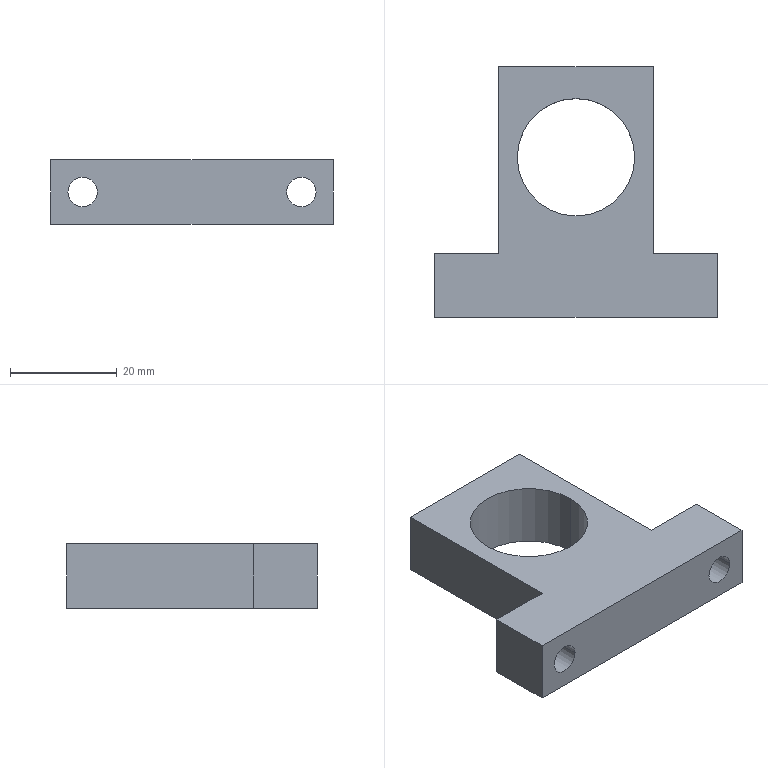Part | SolidWorks | features ICE 2, Extrusion 1 | 1 solid | 22 faces | box 53 x 47 x 12 mm | volume 14045 mm3 | plane 12 | cylinder 10 | commonest cylinder face diameters 5.5 x4 10 x4 22 x2
STEP:
#1=CARTESIAN_POINT('',(-5.27,-9.838,6.));
#2=VERTEX_POINT('',#1);
#3=CARTESIAN_POINT('',(-15.27,-9.838,6.));
#4=VERTEX_POINT('',#3);
#5=CARTESIAN_POINT('',(-10.27,-9.838,6.));
#6=DIRECTION('',(0.,1.,0.));
#7=DIRECTION('',(-1.,0.,0.));
#8=AXIS2_PLACEMENT_3D('',#5,#6,#7);
#9=CIRCLE('',#8,5.);
#10=EDGE_CURVE('',#2,#4,#9,.T.);
#11=ORIENTED_EDGE('',*,*,#10,.F.);
#12=CARTESIAN_POINT('',(-5.27,-4.038,6.));
#13=VERTEX_POINT('',#12);
#14=CARTESIAN_POINT('',(-5.27,-9.838,6.));
#15=DIRECTION('',(0.,1.,0.));
#16=VECTOR('',#15,1000.);
#17=LINE('',#14,#16);
#18=EDGE_CURVE('',#2,#13,#17,.T.);
#19=ORIENTED_EDGE('',*,*,#18,.T.);
#20=CARTESIAN_POINT('',(-15.27,-4.038,6.));
#21=VERTEX_POINT('',#20);
#22=CARTESIAN_POINT('',(-10.27,-4.038,6.));
#23=DIRECTION('',(0.,1.,0.));
#24=DIRECTION('',(-1.,0.,0.));
#25=AXIS2_PLACEMENT_3D('',#22,#23,#24);
#26=CIRCLE('',#25,5.);
#27=EDGE_CURVE('',#13,#21,#26,.T.);
#28=ORIENTED_EDGE('',*,*,#27,.T.);
#29=CARTESIAN_POINT('',(-15.27,-9.838,6.));
#30=DIRECTION('',(0.,1.,0.));
#31=VECTOR('',#30,1000.);
#32=LINE('',#29,#31);
#33=EDGE_CURVE('',#4,#21,#32,.T.);
#34=ORIENTED_EDGE('',*,*,#33,.F.);
#35=EDGE_LOOP('',(#11,#19,#28,#34));
#36=FACE_OUTER_BOUND('',#35,.T.);
#37=CARTESIAN_POINT('',(-10.27,-9.838,6.));
#38=DIRECTION('',(0.,1.,0.));
#39=DIRECTION('',(-1.,0.,0.));
#40=AXIS2_PLACEMENT_3D('',#37,#38,#39);
#41=CYLINDRICAL_SURFACE('',#40,5.);
#42=ADVANCED_FACE('',(#36),#41,.F.);
#43=CARTESIAN_POINT('',(35.73,-9.838,6.));
#44=VERTEX_POINT('',#43);
#45=CARTESIAN_POINT('',(25.73,-9.838,6.));
#46=VERTEX_POINT('',#45);
#47=CARTESIAN_POINT('',(30.73,-9.838,6.));
#48=DIRECTION('',(0.,1.,0.));
#49=DIRECTION('',(-1.,0.,0.));
#50=AXIS2_PLACEMENT_3D('',#47,#48,#49);
#51=CIRCLE('',#50,5.);
#52=EDGE_CURVE('',#44,#46,#51,.T.);
#53=ORIENTED_EDGE('',*,*,#52,.F.);
#54=CARTESIAN_POINT('',(35.73,-4.038,6.));
#55=VERTEX_POINT('',#54);
#56=CARTESIAN_POINT('',(35.73,-9.838,6.));
#57=DIRECTION('',(0.,1.,0.));
#58=VECTOR('',#57,1000.);
#59=LINE('',#56,#58);
#60=EDGE_CURVE('',#44,#55,#59,.T.);
#61=ORIENTED_EDGE('',*,*,#60,.T.);
#62=CARTESIAN_POINT('',(25.73,-4.038,6.));
#63=VERTEX_POINT('',#62);
#64=CARTESIAN_POINT('',(30.73,-4.038,6.));
#65=DIRECTION('',(0.,1.,0.));
#66=DIRECTION('',(-1.,0.,0.));
#67=AXIS2_PLACEMENT_3D('',#64,#65,#66);
#68=CIRCLE('',#67,5.);
#69=EDGE_CURVE('',#55,#63,#68,.T.);
#70=ORIENTED_EDGE('',*,*,#69,.T.);
#71=CARTESIAN_POINT('',(25.73,-9.838,6.));
#72=DIRECTION('',(0.,1.,0.));
#73=VECTOR('',#72,1000.);
#74=LINE('',#71,#73);
#75=EDGE_CURVE('',#46,#63,#74,.T.);
#76=ORIENTED_EDGE('',*,*,#75,.F.);
#77=EDGE_LOOP('',(#53,#61,#70,#76));
#78=FACE_OUTER_BOUND('',#77,.T.);
#79=CARTESIAN_POINT('',(30.73,-9.838,6.));
#80=DIRECTION('',(0.,1.,0.));
#81=DIRECTION('',(-1.,0.,0.));
#82=AXIS2_PLACEMENT_3D('',#79,#80,#81);
#83=CYLINDRICAL_SURFACE('',#82,5.);
#84=ADVANCED_FACE('',(#78),#83,.F.);
#85=CARTESIAN_POINT('',(-0.7697,13.962,12.));
#86=VERTEX_POINT('',#85);
#87=CARTESIAN_POINT('',(21.23,13.962,12.));
#88=VERTEX_POINT('',#87);
#89=CARTESIAN_POINT('',(10.23,13.962,12.));
#90=DIRECTION('',(0.,0.,1.));
#91=DIRECTION('',(1.,0.,0.));
#92=AXIS2_PLACEMENT_3D('',#89,#90,#91);
#93=CIRCLE('',#92,11.);
#94=EDGE_CURVE('',#86,#88,#93,.T.);
#95=ORIENTED_EDGE('',*,*,#94,.T.);
#96=CARTESIAN_POINT('',(21.23,13.962,0.));
#97=VERTEX_POINT('',#96);
#98=CARTESIAN_POINT('',(21.23,13.962,12.));
#99=DIRECTION('',(0.,0.,-1.));
#100=VECTOR('',#99,1000.);
#101=LINE('',#98,#100);
#102=EDGE_CURVE('',#88,#97,#101,.T.);
#103=ORIENTED_EDGE('',*,*,#102,.T.);
#104=CARTESIAN_POINT('',(-0.7697,13.962,0.));
#105=VERTEX_POINT('',#104);
#106=CARTESIAN_POINT('',(10.23,13.962,0.));
#107=DIRECTION('',(0.,0.,1.));
#108=DIRECTION('',(1.,0.,0.));
#109=AXIS2_PLACEMENT_3D('',#106,#107,#108);
#110=CIRCLE('',#109,11.);
#111=EDGE_CURVE('',#105,#97,#110,.T.);
#112=ORIENTED_EDGE('',*,*,#111,.F.);
#113=CARTESIAN_POINT('',(-0.7697,13.962,12.));
#114=DIRECTION('',(0.,0.,-1.));
#115=VECTOR('',#114,1000.);
#116=LINE('',#113,#115);
#117=EDGE_CURVE('',#86,#105,#116,.T.);
#118=ORIENTED_EDGE('',*,*,#117,.F.);
#119=EDGE_LOOP('',(#95,#103,#112,#118));
#120=FACE_OUTER_BOUND('',#119,.T.);
#121=CARTESIAN_POINT('',(10.23,13.962,12.));
#122=DIRECTION('',(0.,0.,-1.));
#123=DIRECTION('',(-1.,0.,0.));
#124=AXIS2_PLACEMENT_3D('',#121,#122,#123);
#125=CYLINDRICAL_SURFACE('',#124,11.);
#126=ADVANCED_FACE('',(#120),#125,.F.);
#127=CARTESIAN_POINT('',(33.48,-16.038,6.));
#128=VERTEX_POINT('',#127);
#129=CARTESIAN_POINT('',(27.98,-16.038,6.));
#130=VERTEX_POINT('',#129);
#131=CARTESIAN_POINT('',(30.73,-16.038,6.));
#132=DIRECTION('',(0.,1.,0.));
#133=DIRECTION('',(-1.,0.,0.));
#134=AXIS2_PLACEMENT_3D('',#131,#132,#133);
#135=CIRCLE('',#134,2.75);
#136=EDGE_CURVE('',#128,#130,#135,.T.);
#137=ORIENTED_EDGE('',*,*,#136,.F.);
#138=CARTESIAN_POINT('',(33.48,-9.838,6.));
#139=VERTEX_POINT('',#138);
#140=CARTESIAN_POINT('',(33.48,-16.038,6.));
#141=DIRECTION('',(0.,1.,0.));
#142=VECTOR('',#141,1000.);
#143=LINE('',#140,#142);
#144=EDGE_CURVE('',#128,#139,#143,.T.);
#145=ORIENTED_EDGE('',*,*,#144,.T.);
#146=CARTESIAN_POINT('',(27.98,-9.838,6.));
#147=VERTEX_POINT('',#146);
#148=CARTESIAN_POINT('',(30.73,-9.838,6.));
#149=DIRECTION('',(0.,-1.,0.));
#150=DIRECTION('',(-1.,0.,0.));
#151=AXIS2_PLACEMENT_3D('',#148,#149,#150);
#152=CIRCLE('',#151,2.75);
#153=EDGE_CURVE('',#147,#139,#152,.T.);
#154=ORIENTED_EDGE('',*,*,#153,.F.);
#155=CARTESIAN_POINT('',(27.98,-16.038,6.));
#156=DIRECTION('',(0.,1.,0.));
#157=VECTOR('',#156,1000.);
#158=LINE('',#155,#157);
#159=EDGE_CURVE('',#130,#147,#158,.T.);
#160=ORIENTED_EDGE('',*,*,#159,.F.);
#161=EDGE_LOOP('',(#137,#145,#154,#160));
#162=FACE_OUTER_BOUND('',#161,.T.);
#163=CARTESIAN_POINT('',(30.73,-16.038,6.));
#164=DIRECTION('',(0.,1.,0.));
#165=DIRECTION('',(-1.,0.,0.));
#166=AXIS2_PLACEMENT_3D('',#163,#164,#165);
#167=CYLINDRICAL_SURFACE('',#166,2.75);
#168=ADVANCED_FACE('',(#162),#167,.F.);
#169=CARTESIAN_POINT('',(-7.52,-16.038,6.));
#170=VERTEX_POINT('',#169);
#171=CARTESIAN_POINT('',(-13.02,-16.038,6.));
#172=VERTEX_POINT('',#171);
#173=CARTESIAN_POINT('',(-10.27,-16.038,6.));
#174=DIRECTION('',(0.,1.,0.));
#175=DIRECTION('',(-1.,0.,0.));
#176=AXIS2_PLACEMENT_3D('',#173,#174,#175);
#177=CIRCLE('',#176,2.75);
#178=EDGE_CURVE('',#170,#172,#177,.T.);
#179=ORIENTED_EDGE('',*,*,#178,.F.);
#180=CARTESIAN_POINT('',(-7.52,-9.838,6.));
#181=VERTEX_POINT('',#180);
#182=CARTESIAN_POINT('',(-7.52,-16.038,6.));
#183=DIRECTION('',(0.,1.,0.));
#184=VECTOR('',#183,1000.);
#185=LINE('',#182,#184);
#186=EDGE_CURVE('',#170,#181,#185,.T.);
#187=ORIENTED_EDGE('',*,*,#186,.T.);
#188=CARTESIAN_POINT('',(-13.02,-9.838,6.));
#189=VERTEX_POINT('',#188);
#190=CARTESIAN_POINT('',(-10.27,-9.838,6.));
#191=DIRECTION('',(0.,-1.,0.));
#192=DIRECTION('',(-1.,0.,0.));
#193=AXIS2_PLACEMENT_3D('',#190,#191,#192);
#194=CIRCLE('',#193,2.75);
#195=EDGE_CURVE('',#189,#181,#194,.T.);
#196=ORIENTED_EDGE('',*,*,#195,.F.);
#197=CARTESIAN_POINT('',(-13.02,-16.038,6.));
#198=DIRECTION('',(0.,1.,0.));
#199=VECTOR('',#198,1000.);
#200=LINE('',#197,#199);
#201=EDGE_CURVE('',#172,#189,#200,.T.);
#202=ORIENTED_EDGE('',*,*,#201,.F.);
#203=EDGE_LOOP('',(#179,#187,#196,#202));
#204=FACE_OUTER_BOUND('',#203,.T.);
#205=CARTESIAN_POINT('',(-10.27,-16.038,6.));
#206=DIRECTION('',(0.,1.,0.));
#207=DIRECTION('',(-1.,0.,0.));
#208=AXIS2_PLACEMENT_3D('',#205,#206,#207);
#209=CYLINDRICAL_SURFACE('',#208,2.75);
#210=ADVANCED_FACE('',(#204),#209,.F.);
#211=ORIENTED_EDGE('',*,*,#186,.F.);
#212=CARTESIAN_POINT('',(-10.27,-16.038,6.));
#213=DIRECTION('',(0.,1.,0.));
#214=DIRECTION('',(-1.,0.,0.));
#215=AXIS2_PLACEMENT_3D('',#212,#213,#214);
#216=CIRCLE('',#215,2.75);
#217=EDGE_CURVE('',#172,#170,#216,.T.);
#218=ORIENTED_EDGE('',*,*,#217,.F.);
#219=ORIENTED_EDGE('',*,*,#201,.T.);
#220=CARTESIAN_POINT('',(-10.27,-9.838,6.));
#221=DIRECTION('',(0.,-1.,0.));
#222=DIRECTION('',(-1.,0.,0.));
#223=AXIS2_PLACEMENT_3D('',#220,#221,#222);
#224=CIRCLE('',#223,2.75);
#225=EDGE_CURVE('',#181,#189,#224,.T.);
#226=ORIENTED_EDGE('',*,*,#225,.F.);
#227=EDGE_LOOP('',(#211,#218,#219,#226));
#228=FACE_OUTER_BOUND('',#227,.T.);
#229=CARTESIAN_POINT('',(-10.27,-16.038,6.));
#230=DIRECTION('',(0.,1.,0.));
#231=DIRECTION('',(-1.,0.,0.));
#232=AXIS2_PLACEMENT_3D('',#229,#230,#231);
#233=CYLINDRICAL_SURFACE('',#232,2.75);
#234=ADVANCED_FACE('',(#228),#233,.F.);
#235=ORIENTED_EDGE('',*,*,#144,.F.);
#236=CARTESIAN_POINT('',(30.73,-16.038,6.));
#237=DIRECTION('',(0.,1.,0.));
#238=DIRECTION('',(-1.,0.,0.));
#239=AXIS2_PLACEMENT_3D('',#236,#237,#238);
#240=CIRCLE('',#239,2.75);
#241=EDGE_CURVE('',#130,#128,#240,.T.);
#242=ORIENTED_EDGE('',*,*,#241,.F.);
#243=ORIENTED_EDGE('',*,*,#159,.T.);
#244=CARTESIAN_POINT('',(30.73,-9.838,6.));
#245=DIRECTION('',(0.,-1.,0.));
#246=DIRECTION('',(-1.,0.,0.));
#247=AXIS2_PLACEMENT_3D('',#244,#245,#246);
#248=CIRCLE('',#247,2.75);
#249=EDGE_CURVE('',#139,#147,#248,.T.);
#250=ORIENTED_EDGE('',*,*,#249,.F.);
#251=EDGE_LOOP('',(#235,#242,#243,#250));
#252=FACE_OUTER_BOUND('',#251,.T.);
#253=CARTESIAN_POINT('',(30.73,-16.038,6.));
#254=DIRECTION('',(0.,1.,0.));
#255=DIRECTION('',(-1.,0.,0.));
#256=AXIS2_PLACEMENT_3D('',#253,#254,#255);
#257=CYLINDRICAL_SURFACE('',#256,2.75);
#258=ADVANCED_FACE('',(#252),#257,.F.);
#259=CARTESIAN_POINT('',(-16.27,-4.038,12.));
#260=VERTEX_POINT('',#259);
#261=CARTESIAN_POINT('',(-16.27,-16.038,12.));
#262=VERTEX_POINT('',#261);
#263=CARTESIAN_POINT('',(-16.27,-4.038,12.));
#264=DIRECTION('',(0.,-1.,0.));
#265=VECTOR('',#264,1000.);
#266=LINE('',#263,#265);
#267=EDGE_CURVE('',#260,#262,#266,.T.);
#268=ORIENTED_EDGE('',*,*,#267,.T.);
#269=CARTESIAN_POINT('',(36.73,-16.038,12.));
#270=VERTEX_POINT('',#269);
#271=CARTESIAN_POINT('',(-16.27,-16.038,12.));
#272=DIRECTION('',(1.,0.,0.));
#273=VECTOR('',#272,1000.);
#274=LINE('',#271,#273);
#275=EDGE_CURVE('',#262,#270,#274,.T.);
#276=ORIENTED_EDGE('',*,*,#275,.T.);
#277=CARTESIAN_POINT('',(36.73,-4.038,12.));
#278=VERTEX_POINT('',#277);
#279=CARTESIAN_POINT('',(36.73,-16.038,12.));
#280=DIRECTION('',(0.,1.,0.));
#281=VECTOR('',#280,1000.);
#282=LINE('',#279,#281);
#283=EDGE_CURVE('',#270,#278,#282,.T.);
#284=ORIENTED_EDGE('',*,*,#283,.T.);
#285=CARTESIAN_POINT('',(24.73,-4.038,12.));
#286=VERTEX_POINT('',#285);
#287=CARTESIAN_POINT('',(36.73,-4.038,12.));
#288=DIRECTION('',(-1.,0.,0.));
#289=VECTOR('',#288,1000.);
#290=LINE('',#287,#289);
#291=EDGE_CURVE('',#278,#286,#290,.T.);
#292=ORIENTED_EDGE('',*,*,#291,.T.);
#293=CARTESIAN_POINT('',(24.73,30.962,12.));
#294=VERTEX_POINT('',#293);
#295=CARTESIAN_POINT('',(24.73,-4.038,12.));
#296=DIRECTION('',(0.,1.,0.));
#297=VECTOR('',#296,1000.);
#298=LINE('',#295,#297);
#299=EDGE_CURVE('',#286,#294,#298,.T.);
#300=ORIENTED_EDGE('',*,*,#299,.T.);
#301=CARTESIAN_POINT('',(-4.27,30.962,12.));
#302=VERTEX_POINT('',#301);
#303=CARTESIAN_POINT('',(24.73,30.962,12.));
#304=DIRECTION('',(-1.,0.,0.));
#305=VECTOR('',#304,1000.);
#306=LINE('',#303,#305);
#307=EDGE_CURVE('',#294,#302,#306,.T.);
#308=ORIENTED_EDGE('',*,*,#307,.T.);
#309=CARTESIAN_POINT('',(-4.27,-4.038,12.));
#310=VERTEX_POINT('',#309);
#311=CARTESIAN_POINT('',(-4.27,30.962,12.));
#312=DIRECTION('',(0.,-1.,0.));
#313=VECTOR('',#312,1000.);
#314=LINE('',#311,#313);
#315=EDGE_CURVE('',#302,#310,#314,.T.);
#316=ORIENTED_EDGE('',*,*,#315,.T.);
#317=CARTESIAN_POINT('',(-4.27,-4.038,12.));
#318=DIRECTION('',(-1.,0.,0.));
#319=VECTOR('',#318,1000.);
#320=LINE('',#317,#319);
#321=EDGE_CURVE('',#310,#260,#320,.T.);
#322=ORIENTED_EDGE('',*,*,#321,.T.);
#323=EDGE_LOOP('',(#268,#276,#284,#292,#300,#308,#316,#322));
#324=FACE_OUTER_BOUND('',#323,.T.);
#325=ORIENTED_EDGE('',*,*,#94,.F.);
#326=CARTESIAN_POINT('',(10.23,13.962,12.));
#327=DIRECTION('',(0.,0.,1.));
#328=DIRECTION('',(1.,0.,0.));
#329=AXIS2_PLACEMENT_3D('',#326,#327,#328);
#330=CIRCLE('',#329,11.);
#331=EDGE_CURVE('',#88,#86,#330,.T.);
#332=ORIENTED_EDGE('',*,*,#331,.F.);
#333=EDGE_LOOP('',(#325,#332));
#334=FACE_BOUND('',#333,.T.);
#335=CARTESIAN_POINT('',(0.,0.,12.));
#336=DIRECTION('',(0.,0.,1.));
#337=DIRECTION('',(1.,0.,0.));
#338=AXIS2_PLACEMENT_3D('',#335,#336,#337);
#339=PLANE('',#338);
#340=ADVANCED_FACE('',(#324,#334),#339,.T.);
#341=CARTESIAN_POINT('',(-16.27,-4.038,0.));
#342=VERTEX_POINT('',#341);
#343=CARTESIAN_POINT('',(-16.27,-16.038,0.));
#344=VERTEX_POINT('',#343);
#345=CARTESIAN_POINT('',(-16.27,-4.038,0.));
#346=DIRECTION('',(0.,-1.,0.));
#347=VECTOR('',#346,1000.);
#348=LINE('',#345,#347);
#349=EDGE_CURVE('',#342,#344,#348,.T.);
#350=ORIENTED_EDGE('',*,*,#349,.F.);
#351=CARTESIAN_POINT('',(-4.27,-4.038,0.));
#352=VERTEX_POINT('',#351);
#353=CARTESIAN_POINT('',(-4.27,-4.038,0.));
#354=DIRECTION('',(-1.,0.,0.));
#355=VECTOR('',#354,1000.);
#356=LINE('',#353,#355);
#357=EDGE_CURVE('',#352,#342,#356,.T.);
#358=ORIENTED_EDGE('',*,*,#357,.F.);
#359=CARTESIAN_POINT('',(-4.27,30.962,0.));
#360=VERTEX_POINT('',#359);
#361=CARTESIAN_POINT('',(-4.27,30.962,0.));
#362=DIRECTION('',(0.,-1.,0.));
#363=VECTOR('',#362,1000.);
#364=LINE('',#361,#363);
#365=EDGE_CURVE('',#360,#352,#364,.T.);
#366=ORIENTED_EDGE('',*,*,#365,.F.);
#367=CARTESIAN_POINT('',(24.73,30.962,0.));
#368=VERTEX_POINT('',#367);
#369=CARTESIAN_POINT('',(24.73,30.962,0.));
#370=DIRECTION('',(-1.,0.,0.));
#371=VECTOR('',#370,1000.);
#372=LINE('',#369,#371);
#373=EDGE_CURVE('',#368,#360,#372,.T.);
#374=ORIENTED_EDGE('',*,*,#373,.F.);
#375=CARTESIAN_POINT('',(24.73,-4.038,0.));
#376=VERTEX_POINT('',#375);
#377=CARTESIAN_POINT('',(24.73,-4.038,0.));
#378=DIRECTION('',(0.,1.,0.));
#379=VECTOR('',#378,1000.);
#380=LINE('',#377,#379);
#381=EDGE_CURVE('',#376,#368,#380,.T.);
#382=ORIENTED_EDGE('',*,*,#381,.F.);
#383=CARTESIAN_POINT('',(36.73,-4.038,0.));
#384=VERTEX_POINT('',#383);
#385=CARTESIAN_POINT('',(36.73,-4.038,0.));
#386=DIRECTION('',(-1.,0.,0.));
#387=VECTOR('',#386,1000.);
#388=LINE('',#385,#387);
#389=EDGE_CURVE('',#384,#376,#388,.T.);
#390=ORIENTED_EDGE('',*,*,#389,.F.);
#391=CARTESIAN_POINT('',(36.73,-16.038,0.));
#392=VERTEX_POINT('',#391);
#393=CARTESIAN_POINT('',(36.73,-16.038,0.));
#394=DIRECTION('',(0.,1.,0.));
#395=VECTOR('',#394,1000.);
#396=LINE('',#393,#395);
#397=EDGE_CURVE('',#392,#384,#396,.T.);
#398=ORIENTED_EDGE('',*,*,#397,.F.);
#399=CARTESIAN_POINT('',(-16.27,-16.038,0.));
#400=DIRECTION('',(1.,0.,0.));
#401=VECTOR('',#400,1000.);
#402=LINE('',#399,#401);
#403=EDGE_CURVE('',#344,#392,#402,.T.);
#404=ORIENTED_EDGE('',*,*,#403,.F.);
#405=EDGE_LOOP('',(#350,#358,#366,#374,#382,#390,#398,#404));
#406=FACE_OUTER_BOUND('',#405,.T.);
#407=ORIENTED_EDGE('',*,*,#111,.T.);
#408=CARTESIAN_POINT('',(10.23,13.962,0.));
#409=DIRECTION('',(0.,0.,1.));
#410=DIRECTION('',(1.,0.,0.));
#411=AXIS2_PLACEMENT_3D('',#408,#409,#410);
#412=CIRCLE('',#411,11.);
#413=EDGE_CURVE('',#97,#105,#412,.T.);
#414=ORIENTED_EDGE('',*,*,#413,.T.);
#415=EDGE_LOOP('',(#407,#414));
#416=FACE_BOUND('',#415,.T.);
#417=CARTESIAN_POINT('',(0.,0.,0.));
#418=DIRECTION('',(0.,0.,1.));
#419=DIRECTION('',(1.,0.,0.));
#420=AXIS2_PLACEMENT_3D('',#417,#418,#419);
#421=PLANE('',#420);
#422=ADVANCED_FACE('',(#406,#416),#421,.F.);
#423=ORIENTED_EDGE('',*,*,#349,.T.);
#424=CARTESIAN_POINT('',(-16.27,-16.038,12.));
#425=DIRECTION('',(0.,0.,-1.));
#426=VECTOR('',#425,1000.);
#427=LINE('',#424,#426);
#428=EDGE_CURVE('',#262,#344,#427,.T.);
#429=ORIENTED_EDGE('',*,*,#428,.F.);
#430=ORIENTED_EDGE('',*,*,#267,.F.);
#431=CARTESIAN_POINT('',(-16.27,-4.038,12.));
#432=DIRECTION('',(0.,0.,-1.));
#433=VECTOR('',#432,1000.);
#434=LINE('',#431,#433);
#435=EDGE_CURVE('',#260,#342,#434,.T.);
#436=ORIENTED_EDGE('',*,*,#435,.T.);
#437=EDGE_LOOP('',(#423,#429,#430,#436));
#438=FACE_OUTER_BOUND('',#437,.T.);
#439=CARTESIAN_POINT('',(-16.27,-4.038,12.));
#440=DIRECTION('',(1.,0.,0.));
#441=DIRECTION('',(0.,1.,0.));
#442=AXIS2_PLACEMENT_3D('',#439,#440,#441);
#443=PLANE('',#442);
#444=ADVANCED_FACE('',(#438),#443,.F.);
#445=ORIENTED_EDGE('',*,*,#217,.T.);
#446=ORIENTED_EDGE('',*,*,#178,.T.);
#447=EDGE_LOOP('',(#445,#446));
#448=FACE_BOUND('',#447,.T.);
#449=ORIENTED_EDGE('',*,*,#241,.T.);
#450=ORIENTED_EDGE('',*,*,#136,.T.);
#451=EDGE_LOOP('',(#449,#450));
#452=FACE_BOUND('',#451,.T.);
#453=ORIENTED_EDGE('',*,*,#403,.T.);
#454=CARTESIAN_POINT('',(36.73,-16.038,12.));
#455=DIRECTION('',(0.,0.,-1.));
#456=VECTOR('',#455,1000.);
#457=LINE('',#454,#456);
#458=EDGE_CURVE('',#270,#392,#457,.T.);
#459=ORIENTED_EDGE('',*,*,#458,.F.);
#460=ORIENTED_EDGE('',*,*,#275,.F.);
#461=ORIENTED_EDGE('',*,*,#428,.T.);
#462=EDGE_LOOP('',(#453,#459,#460,#461));
#463=FACE_OUTER_BOUND('',#462,.T.);
#464=CARTESIAN_POINT('',(-16.27,-16.038,12.));
#465=DIRECTION('',(0.,1.,0.));
#466=DIRECTION('',(-1.,0.,0.));
#467=AXIS2_PLACEMENT_3D('',#464,#465,#466);
#468=PLANE('',#467);
#469=ADVANCED_FACE('',(#448,#452,#463),#468,.F.);
#470=ORIENTED_EDGE('',*,*,#397,.T.);
#471=CARTESIAN_POINT('',(36.73,-4.038,12.));
#472=DIRECTION('',(0.,0.,-1.));
#473=VECTOR('',#472,1000.);
#474=LINE('',#471,#473);
#475=EDGE_CURVE('',#278,#384,#474,.T.);
#476=ORIENTED_EDGE('',*,*,#475,.F.);
#477=ORIENTED_EDGE('',*,*,#283,.F.);
#478=ORIENTED_EDGE('',*,*,#458,.T.);
#479=EDGE_LOOP('',(#470,#476,#477,#478));
#480=FACE_OUTER_BOUND('',#479,.T.);
#481=CARTESIAN_POINT('',(36.73,-16.038,12.));
#482=DIRECTION('',(-1.,0.,0.));
#483=DIRECTION('',(0.,0.,1.));
#484=AXIS2_PLACEMENT_3D('',#481,#482,#483);
#485=PLANE('',#484);
#486=ADVANCED_FACE('',(#480),#485,.F.);
#487=CARTESIAN_POINT('',(30.73,-4.038,6.));
#488=DIRECTION('',(0.,1.,0.));
#489=DIRECTION('',(-1.,0.,0.));
#490=AXIS2_PLACEMENT_3D('',#487,#488,#489);
#491=CIRCLE('',#490,5.);
#492=EDGE_CURVE('',#63,#55,#491,.T.);
#493=ORIENTED_EDGE('',*,*,#492,.F.);
#494=ORIENTED_EDGE('',*,*,#69,.F.);
#495=EDGE_LOOP('',(#493,#494));
#496=FACE_BOUND('',#495,.T.);
#497=ORIENTED_EDGE('',*,*,#389,.T.);
#498=CARTESIAN_POINT('',(24.73,-4.038,12.));
#499=DIRECTION('',(0.,0.,-1.));
#500=VECTOR('',#499,1000.);
#501=LINE('',#498,#500);
#502=EDGE_CURVE('',#286,#376,#501,.T.);
#503=ORIENTED_EDGE('',*,*,#502,.F.);
#504=ORIENTED_EDGE('',*,*,#291,.F.);
#505=ORIENTED_EDGE('',*,*,#475,.T.);
#506=EDGE_LOOP('',(#497,#503,#504,#505));
#507=FACE_OUTER_BOUND('',#506,.T.);
#508=CARTESIAN_POINT('',(36.73,-4.038,12.));
#509=DIRECTION('',(0.,-1.,0.));
#510=DIRECTION('',(1.,0.,0.));
#511=AXIS2_PLACEMENT_3D('',#508,#509,#510);
#512=PLANE('',#511);
#513=ADVANCED_FACE('',(#496,#507),#512,.F.);
#514=ORIENTED_EDGE('',*,*,#381,.T.);
#515=CARTESIAN_POINT('',(24.73,30.962,12.));
#516=DIRECTION('',(0.,0.,-1.));
#517=VECTOR('',#516,1000.);
#518=LINE('',#515,#517);
#519=EDGE_CURVE('',#294,#368,#518,.T.);
#520=ORIENTED_EDGE('',*,*,#519,.F.);
#521=ORIENTED_EDGE('',*,*,#299,.F.);
#522=ORIENTED_EDGE('',*,*,#502,.T.);
#523=EDGE_LOOP('',(#514,#520,#521,#522));
#524=FACE_OUTER_BOUND('',#523,.T.);
#525=CARTESIAN_POINT('',(24.73,-4.038,12.));
#526=DIRECTION('',(-1.,0.,0.));
#527=DIRECTION('',(0.,0.,1.));
#528=AXIS2_PLACEMENT_3D('',#525,#526,#527);
#529=PLANE('',#528);
#530=ADVANCED_FACE('',(#524),#529,.F.);
#531=ORIENTED_EDGE('',*,*,#373,.T.);
#532=CARTESIAN_POINT('',(-4.27,30.962,12.));
#533=DIRECTION('',(0.,0.,-1.));
#534=VECTOR('',#533,1000.);
#535=LINE('',#532,#534);
#536=EDGE_CURVE('',#302,#360,#535,.T.);
#537=ORIENTED_EDGE('',*,*,#536,.F.);
#538=ORIENTED_EDGE('',*,*,#307,.F.);
#539=ORIENTED_EDGE('',*,*,#519,.T.);
#540=EDGE_LOOP('',(#531,#537,#538,#539));
#541=FACE_OUTER_BOUND('',#540,.T.);
#542=CARTESIAN_POINT('',(24.73,30.962,12.));
#543=DIRECTION('',(0.,-1.,0.));
#544=DIRECTION('',(1.,0.,0.));
#545=AXIS2_PLACEMENT_3D('',#542,#543,#544);
#546=PLANE('',#545);
#547=ADVANCED_FACE('',(#541),#546,.F.);
#548=ORIENTED_EDGE('',*,*,#365,.T.);
#549=CARTESIAN_POINT('',(-4.27,-4.038,12.));
#550=DIRECTION('',(0.,0.,-1.));
#551=VECTOR('',#550,1000.);
#552=LINE('',#549,#551);
#553=EDGE_CURVE('',#310,#352,#552,.T.);
#554=ORIENTED_EDGE('',*,*,#553,.F.);
#555=ORIENTED_EDGE('',*,*,#315,.F.);
#556=ORIENTED_EDGE('',*,*,#536,.T.);
#557=EDGE_LOOP('',(#548,#554,#555,#556));
#558=FACE_OUTER_BOUND('',#557,.T.);
#559=CARTESIAN_POINT('',(-4.27,30.962,12.));
#560=DIRECTION('',(1.,0.,0.));
#561=DIRECTION('',(0.,1.,0.));
#562=AXIS2_PLACEMENT_3D('',#559,#560,#561);
#563=PLANE('',#562);
#564=ADVANCED_FACE('',(#558),#563,.F.);
#565=CARTESIAN_POINT('',(-10.27,-4.038,6.));
#566=DIRECTION('',(0.,1.,0.));
#567=DIRECTION('',(-1.,0.,0.));
#568=AXIS2_PLACEMENT_3D('',#565,#566,#567);
#569=CIRCLE('',#568,5.);
#570=EDGE_CURVE('',#21,#13,#569,.T.);
#571=ORIENTED_EDGE('',*,*,#570,.F.);
#572=ORIENTED_EDGE('',*,*,#27,.F.);
#573=EDGE_LOOP('',(#571,#572));
#574=FACE_BOUND('',#573,.T.);
#575=ORIENTED_EDGE('',*,*,#357,.T.);
#576=ORIENTED_EDGE('',*,*,#435,.F.);
#577=ORIENTED_EDGE('',*,*,#321,.F.);
#578=ORIENTED_EDGE('',*,*,#553,.T.);
#579=EDGE_LOOP('',(#575,#576,#577,#578));
#580=FACE_OUTER_BOUND('',#579,.T.);
#581=CARTESIAN_POINT('',(-4.27,-4.038,12.));
#582=DIRECTION('',(0.,-1.,0.));
#583=DIRECTION('',(1.,0.,0.));
#584=AXIS2_PLACEMENT_3D('',#581,#582,#583);
#585=PLANE('',#584);
#586=ADVANCED_FACE('',(#574,#580),#585,.F.);
#587=ORIENTED_EDGE('',*,*,#102,.F.);
#588=ORIENTED_EDGE('',*,*,#331,.T.);
#589=ORIENTED_EDGE('',*,*,#117,.T.);
#590=ORIENTED_EDGE('',*,*,#413,.F.);
#591=EDGE_LOOP('',(#587,#588,#589,#590));
#592=FACE_OUTER_BOUND('',#591,.T.);
#593=CARTESIAN_POINT('',(10.23,13.962,12.));
#594=DIRECTION('',(0.,0.,-1.));
#595=DIRECTION('',(-1.,0.,0.));
#596=AXIS2_PLACEMENT_3D('',#593,#594,#595);
#597=CYLINDRICAL_SURFACE('',#596,11.);
#598=ADVANCED_FACE('',(#592),#597,.F.);
#599=CARTESIAN_POINT('',(30.73,-9.838,6.));
#600=DIRECTION('',(0.,1.,0.));
#601=DIRECTION('',(-1.,0.,0.));
#602=AXIS2_PLACEMENT_3D('',#599,#600,#601);
#603=CIRCLE('',#602,5.);
#604=EDGE_CURVE('',#46,#44,#603,.T.);
#605=ORIENTED_EDGE('',*,*,#604,.T.);
#606=ORIENTED_EDGE('',*,*,#52,.T.);
#607=EDGE_LOOP('',(#605,#606));
#608=FACE_OUTER_BOUND('',#607,.T.);
#609=ORIENTED_EDGE('',*,*,#153,.T.);
#610=ORIENTED_EDGE('',*,*,#249,.T.);
#611=EDGE_LOOP('',(#609,#610));
#612=FACE_BOUND('',#611,.T.);
#613=CARTESIAN_POINT('',(30.73,-9.838,6.));
#614=DIRECTION('',(0.,1.,0.));
#615=DIRECTION('',(-1.,0.,0.));
#616=AXIS2_PLACEMENT_3D('',#613,#614,#615);
#617=PLANE('',#616);
#618=ADVANCED_FACE('',(#608,#612),#617,.T.);
#619=ORIENTED_EDGE('',*,*,#60,.F.);
#620=ORIENTED_EDGE('',*,*,#604,.F.);
#621=ORIENTED_EDGE('',*,*,#75,.T.);
#622=ORIENTED_EDGE('',*,*,#492,.T.);
#623=EDGE_LOOP('',(#619,#620,#621,#622));
#624=FACE_OUTER_BOUND('',#623,.T.);
#625=CARTESIAN_POINT('',(30.73,-9.838,6.));
#626=DIRECTION('',(0.,1.,0.));
#627=DIRECTION('',(-1.,0.,0.));
#628=AXIS2_PLACEMENT_3D('',#625,#626,#627);
#629=CYLINDRICAL_SURFACE('',#628,5.);
#630=ADVANCED_FACE('',(#624),#629,.F.);
#631=CARTESIAN_POINT('',(-10.27,-9.838,6.));
#632=DIRECTION('',(0.,1.,0.));
#633=DIRECTION('',(-1.,0.,0.));
#634=AXIS2_PLACEMENT_3D('',#631,#632,#633);
#635=CIRCLE('',#634,5.);
#636=EDGE_CURVE('',#4,#2,#635,.T.);
#637=ORIENTED_EDGE('',*,*,#636,.T.);
#638=ORIENTED_EDGE('',*,*,#10,.T.);
#639=EDGE_LOOP('',(#637,#638));
#640=FACE_OUTER_BOUND('',#639,.T.);
#641=ORIENTED_EDGE('',*,*,#195,.T.);
#642=ORIENTED_EDGE('',*,*,#225,.T.);
#643=EDGE_LOOP('',(#641,#642));
#644=FACE_BOUND('',#643,.T.);
#645=CARTESIAN_POINT('',(-10.27,-9.838,6.));
#646=DIRECTION('',(0.,1.,0.));
#647=DIRECTION('',(-1.,0.,0.));
#648=AXIS2_PLACEMENT_3D('',#645,#646,#647);
#649=PLANE('',#648);
#650=ADVANCED_FACE('',(#640,#644),#649,.T.);
#651=ORIENTED_EDGE('',*,*,#18,.F.);
#652=ORIENTED_EDGE('',*,*,#636,.F.);
#653=ORIENTED_EDGE('',*,*,#33,.T.);
#654=ORIENTED_EDGE('',*,*,#570,.T.);
#655=EDGE_LOOP('',(#651,#652,#653,#654));
#656=FACE_OUTER_BOUND('',#655,.T.);
#657=CARTESIAN_POINT('',(-10.27,-9.838,6.));
#658=DIRECTION('',(0.,1.,0.));
#659=DIRECTION('',(-1.,0.,0.));
#660=AXIS2_PLACEMENT_3D('',#657,#658,#659);
#661=CYLINDRICAL_SURFACE('',#660,5.);
#662=ADVANCED_FACE('',(#656),#661,.F.);
#663=CLOSED_SHELL('',(#42,#84,#126,#168,#210,#234,#258,#340,#422,#444,#469,#486,#513,#530,#547,#564,#586,#598,#618,#630,#650,#662));
#664=MANIFOLD_SOLID_BREP('',#663);
#665=CARTESIAN_POINT('',(0.,0.,0.));
#666=DIRECTION('',(0.,0.,1.));
#667=DIRECTION('',(1.,0.,0.));
#668=AXIS2_PLACEMENT_3D('',#665,#666,#667);
#669=(LENGTH_UNIT()NAMED_UNIT(*)SI_UNIT(.MILLI.,.METRE.));
#670=UNCERTAINTY_MEASURE_WITH_UNIT(LENGTH_MEASURE(0.00001),#669,'','');
#671=(NAMED_UNIT(*)PLANE_ANGLE_UNIT()SI_UNIT($,.RADIAN.));
#672=(NAMED_UNIT(*)SI_UNIT($,.STERADIAN.)SOLID_ANGLE_UNIT());
#673=(GEOMETRIC_REPRESENTATION_CONTEXT(3)GLOBAL_UNCERTAINTY_ASSIGNED_CONTEXT((#670))GLOBAL_UNIT_ASSIGNED_CONTEXT((#669,#671,#672))REPRESENTATION_CONTEXT('',''));
#674=ADVANCED_BREP_SHAPE_REPRESENTATION('',(#664,#668),#673);